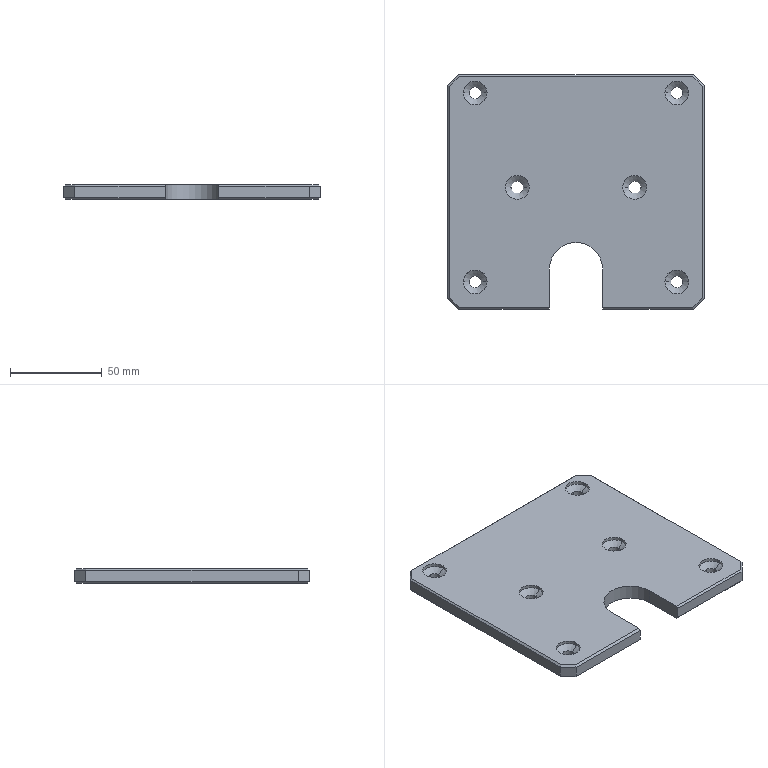Part | Creo | 1 solid | 68 faces | box 140 x 128 x 8 mm | volume 131202 mm3 | plane 31 | cylinder 25 | cone 12 | commonest cylinder face diameters 6.6 x12 13 x12 29 x1